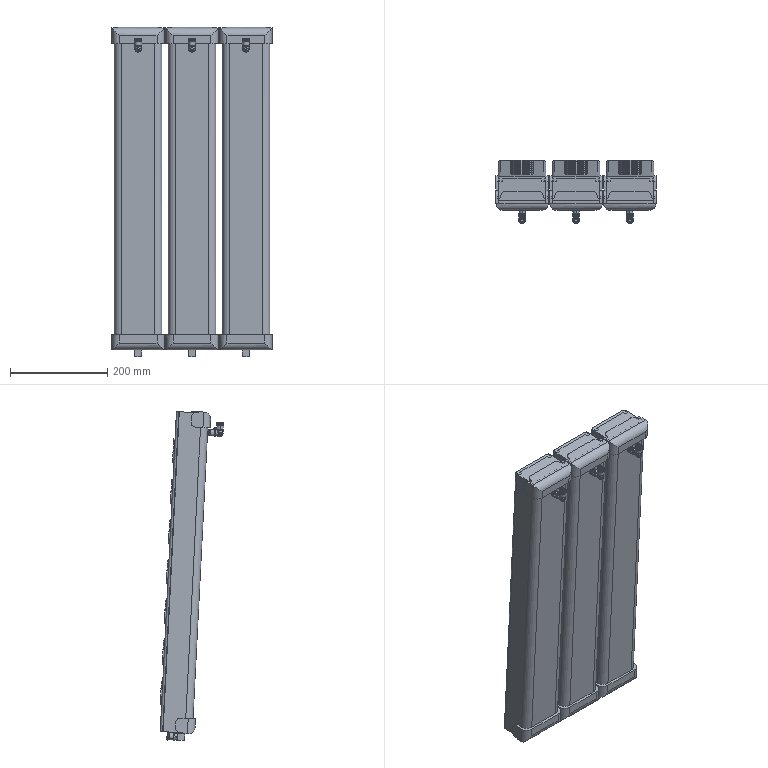Part | SolidWorks | 72 solids | 4254 faces | volume 4563696 mm3 | plane 2349 | cylinder 1296 | cone 378 | torus 120 | spline 81 | sphere 30 | commonest cylinder face diameters 10.222 x168 30.787 x168 8.17 x84 6.779 x72 30 x60 7.866 x57